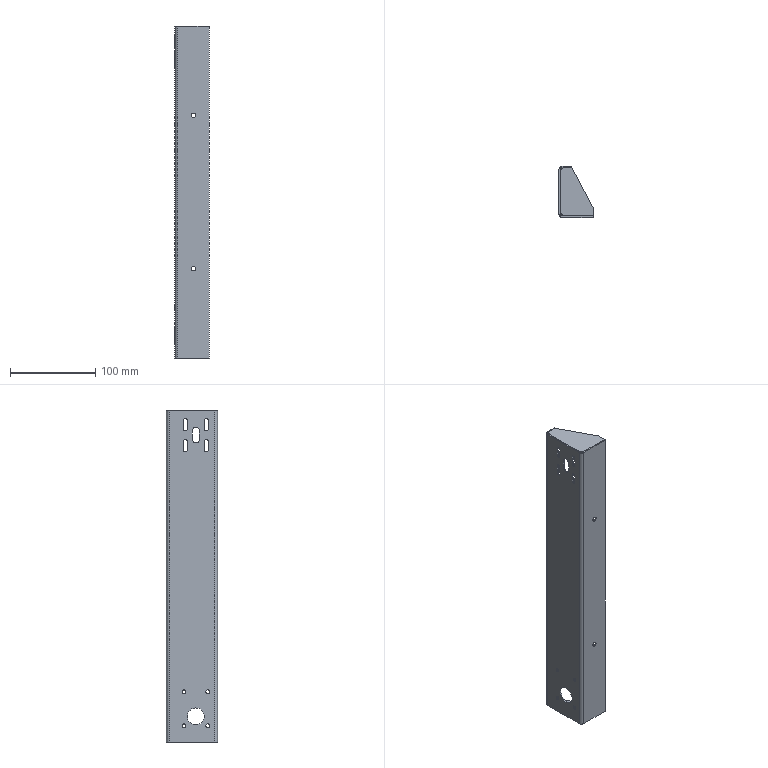Part | SolidWorks | features BaseBody 3 | 3 solids | 87 faces | box 40 x 60 x 390 mm | volume 67667 mm3 | plane 46 | cylinder 41 | commonest cylinder face diameters 4.5 x20 2.5 x8 5.5 x4 8.5 x3 4 x2 7 x2